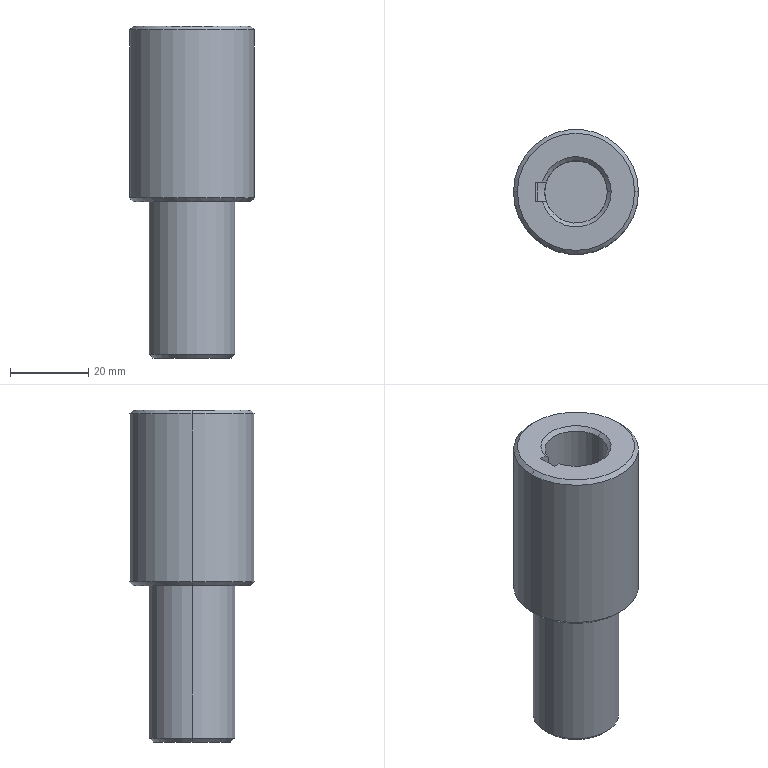Part | STEP file | HXGR200008-05-12-03 | 1 solid | 23 faces | box 32 x 32 x 85 mm | volume 43804 mm3 | cone 9 | plane 8 | cylinder 6 | commonest cylinder face diameters 16 x2 22 x2 32 x2
STEP:
#1=CARTESIAN_POINT('',(-10.,0.,0.));
#2=VERTEX_POINT('',#1);
#3=CARTESIAN_POINT('',(10.,0.,0.));
#4=VERTEX_POINT('',#3);
#5=CARTESIAN_POINT('',(0.,0.,0.));
#6=DIRECTION('',(0.,0.,-1.));
#7=DIRECTION('',(1.,0.,0.));
#8=AXIS2_PLACEMENT_3D('',#5,#6,#7);
#9=CIRCLE('',#8,10.);
#10=EDGE_CURVE('',#2,#4,#9,.T.);
#11=ORIENTED_EDGE('',*,*,#10,.F.);
#12=CARTESIAN_POINT('',(-11.,0.,1.));
#13=VERTEX_POINT('',#12);
#14=CARTESIAN_POINT('',(-11.,0.,1.));
#15=DIRECTION('',(-0.7071,0.,0.7071));
#16=VECTOR('',#15,1000.);
#17=LINE('',#14,#16);
#18=EDGE_CURVE('',#2,#13,#17,.T.);
#19=ORIENTED_EDGE('',*,*,#18,.T.);
#20=CARTESIAN_POINT('',(11.,0.,1.));
#21=VERTEX_POINT('',#20);
#22=CARTESIAN_POINT('',(0.,0.,1.));
#23=DIRECTION('',(0.,0.,1.));
#24=DIRECTION('',(1.,0.,0.));
#25=AXIS2_PLACEMENT_3D('',#22,#23,#24);
#26=CIRCLE('',#25,11.);
#27=EDGE_CURVE('',#21,#13,#26,.T.);
#28=ORIENTED_EDGE('',*,*,#27,.F.);
#29=CARTESIAN_POINT('',(11.,0.,1.));
#30=DIRECTION('',(0.7071,0.,0.7071));
#31=VECTOR('',#30,1000.);
#32=LINE('',#29,#31);
#33=EDGE_CURVE('',#4,#21,#32,.T.);
#34=ORIENTED_EDGE('',*,*,#33,.F.);
#35=EDGE_LOOP('',(#11,#19,#28,#34));
#36=FACE_OUTER_BOUND('',#35,.T.);
#37=CARTESIAN_POINT('',(0.,0.,1.));
#38=DIRECTION('',(0.,0.,1.));
#39=DIRECTION('',(1.,0.,0.));
#40=AXIS2_PLACEMENT_3D('',#37,#38,#39);
#41=CONICAL_SURFACE('',#40,11.,0.7854);
#42=ADVANCED_FACE('',(#36),#41,.T.);
#43=CARTESIAN_POINT('',(-15.,0.,40.));
#44=VERTEX_POINT('',#43);
#45=CARTESIAN_POINT('',(15.,0.,40.));
#46=VERTEX_POINT('',#45);
#47=CARTESIAN_POINT('',(0.,0.,40.));
#48=DIRECTION('',(0.,0.,-1.));
#49=DIRECTION('',(1.,0.,0.));
#50=AXIS2_PLACEMENT_3D('',#47,#48,#49);
#51=CIRCLE('',#50,15.);
#52=EDGE_CURVE('',#44,#46,#51,.T.);
#53=ORIENTED_EDGE('',*,*,#52,.F.);
#54=CARTESIAN_POINT('',(-16.,0.,41.));
#55=VERTEX_POINT('',#54);
#56=CARTESIAN_POINT('',(-16.,0.,41.));
#57=DIRECTION('',(-0.7071,0.,0.7071));
#58=VECTOR('',#57,1000.);
#59=LINE('',#56,#58);
#60=EDGE_CURVE('',#44,#55,#59,.T.);
#61=ORIENTED_EDGE('',*,*,#60,.T.);
#62=CARTESIAN_POINT('',(16.,0.,41.));
#63=VERTEX_POINT('',#62);
#64=CARTESIAN_POINT('',(0.,0.,41.));
#65=DIRECTION('',(0.,0.,1.));
#66=DIRECTION('',(1.,0.,0.));
#67=AXIS2_PLACEMENT_3D('',#64,#65,#66);
#68=CIRCLE('',#67,16.);
#69=EDGE_CURVE('',#63,#55,#68,.T.);
#70=ORIENTED_EDGE('',*,*,#69,.F.);
#71=CARTESIAN_POINT('',(16.,0.,41.));
#72=DIRECTION('',(0.7071,0.,0.7071));
#73=VECTOR('',#72,1000.);
#74=LINE('',#71,#73);
#75=EDGE_CURVE('',#46,#63,#74,.T.);
#76=ORIENTED_EDGE('',*,*,#75,.F.);
#77=EDGE_LOOP('',(#53,#61,#70,#76));
#78=FACE_OUTER_BOUND('',#77,.T.);
#79=CARTESIAN_POINT('',(0.,0.,41.));
#80=DIRECTION('',(0.,0.,1.));
#81=DIRECTION('',(1.,0.,0.));
#82=AXIS2_PLACEMENT_3D('',#79,#80,#81);
#83=CONICAL_SURFACE('',#82,16.,0.7854);
#84=ADVANCED_FACE('',(#78),#83,.T.);
#85=CARTESIAN_POINT('',(15.,0.,85.));
#86=VERTEX_POINT('',#85);
#87=CARTESIAN_POINT('',(-15.,0.,85.));
#88=VERTEX_POINT('',#87);
#89=CARTESIAN_POINT('',(0.,0.,85.));
#90=DIRECTION('',(0.,0.,1.));
#91=DIRECTION('',(1.,0.,0.));
#92=AXIS2_PLACEMENT_3D('',#89,#90,#91);
#93=CIRCLE('',#92,15.);
#94=EDGE_CURVE('',#86,#88,#93,.T.);
#95=ORIENTED_EDGE('',*,*,#94,.F.);
#96=CARTESIAN_POINT('',(16.,0.,84.));
#97=VERTEX_POINT('',#96);
#98=CARTESIAN_POINT('',(15.,0.,85.));
#99=DIRECTION('',(0.7071,0.,-0.7071));
#100=VECTOR('',#99,1000.);
#101=LINE('',#98,#100);
#102=EDGE_CURVE('',#86,#97,#101,.T.);
#103=ORIENTED_EDGE('',*,*,#102,.T.);
#104=CARTESIAN_POINT('',(-16.,0.,84.));
#105=VERTEX_POINT('',#104);
#106=CARTESIAN_POINT('',(0.,0.,84.));
#107=DIRECTION('',(0.,0.,-1.));
#108=DIRECTION('',(1.,0.,0.));
#109=AXIS2_PLACEMENT_3D('',#106,#107,#108);
#110=CIRCLE('',#109,16.);
#111=EDGE_CURVE('',#105,#97,#110,.T.);
#112=ORIENTED_EDGE('',*,*,#111,.F.);
#113=CARTESIAN_POINT('',(-15.,0.,85.));
#114=DIRECTION('',(-0.7071,0.,-0.7071));
#115=VECTOR('',#114,1000.);
#116=LINE('',#113,#115);
#117=EDGE_CURVE('',#88,#105,#116,.T.);
#118=ORIENTED_EDGE('',*,*,#117,.F.);
#119=EDGE_LOOP('',(#95,#103,#112,#118));
#120=FACE_OUTER_BOUND('',#119,.T.);
#121=CARTESIAN_POINT('',(0.,0.,85.));
#122=DIRECTION('',(0.,0.,-1.));
#123=DIRECTION('',(-1.,0.,0.));
#124=AXIS2_PLACEMENT_3D('',#121,#122,#123);
#125=CONICAL_SURFACE('',#124,15.,0.7854);
#126=ADVANCED_FACE('',(#120),#125,.T.);
#127=CARTESIAN_POINT('',(8.,0.,84.));
#128=VERTEX_POINT('',#127);
#129=CARTESIAN_POINT('',(-7.599,2.5,84.));
#130=VERTEX_POINT('',#129);
#131=CARTESIAN_POINT('',(0.,0.,84.));
#132=DIRECTION('',(0.,0.,1.));
#133=DIRECTION('',(1.,0.,0.));
#134=AXIS2_PLACEMENT_3D('',#131,#132,#133);
#135=CIRCLE('',#134,8.);
#136=EDGE_CURVE('',#128,#130,#135,.T.);
#137=ORIENTED_EDGE('',*,*,#136,.F.);
#138=CARTESIAN_POINT('',(9.,0.,85.));
#139=VERTEX_POINT('',#138);
#140=CARTESIAN_POINT('',(8.,0.,84.));
#141=DIRECTION('',(0.7071,0.,0.7071));
#142=VECTOR('',#141,1000.);
#143=LINE('',#140,#142);
#144=EDGE_CURVE('',#128,#139,#143,.T.);
#145=ORIENTED_EDGE('',*,*,#144,.T.);
#146=CARTESIAN_POINT('',(-8.646,2.5,85.));
#147=VERTEX_POINT('',#146);
#148=CARTESIAN_POINT('',(0.,0.,85.));
#149=DIRECTION('',(0.,0.,-1.));
#150=DIRECTION('',(1.,0.,0.));
#151=AXIS2_PLACEMENT_3D('',#148,#149,#150);
#152=CIRCLE('',#151,9.);
#153=EDGE_CURVE('',#147,#139,#152,.T.);
#154=ORIENTED_EDGE('',*,*,#153,.F.);
#155=CARTESIAN_POINT('',(-7.599,2.5,84.));
#156=CARTESIAN_POINT('',(-7.949,2.5,84.332));
#157=CARTESIAN_POINT('',(-8.298,2.5,84.666));
#158=CARTESIAN_POINT('',(-8.646,2.5,85.));
#159=B_SPLINE_CURVE_WITH_KNOTS('',3,(#155,#156,#157,#158),.UNSPECIFIED.,.F.,.F.,(4,4),(0.008066,0.009509),.UNSPECIFIED.);
#160=EDGE_CURVE('',#130,#147,#159,.T.);
#161=ORIENTED_EDGE('',*,*,#160,.F.);
#162=EDGE_LOOP('',(#137,#145,#154,#161));
#163=FACE_OUTER_BOUND('',#162,.T.);
#164=CARTESIAN_POINT('',(0.,0.,84.));
#165=DIRECTION('',(0.,0.,1.));
#166=DIRECTION('',(1.,0.,0.));
#167=AXIS2_PLACEMENT_3D('',#164,#165,#166);
#168=CONICAL_SURFACE('',#167,8.,0.7854);
#169=ADVANCED_FACE('',(#163),#168,.F.);
#170=CARTESIAN_POINT('',(-8.,0.,50.));
#171=VERTEX_POINT('',#170);
#172=CARTESIAN_POINT('',(8.,0.,50.));
#173=VERTEX_POINT('',#172);
#174=CARTESIAN_POINT('',(0.,0.,50.));
#175=DIRECTION('',(0.,0.,1.));
#176=DIRECTION('',(1.,0.,0.));
#177=AXIS2_PLACEMENT_3D('',#174,#175,#176);
#178=CIRCLE('',#177,8.);
#179=EDGE_CURVE('',#171,#173,#178,.T.);
#180=ORIENTED_EDGE('',*,*,#179,.F.);
#181=CARTESIAN_POINT('',(-8.,0.,51.));
#182=VERTEX_POINT('',#181);
#183=CARTESIAN_POINT('',(-8.,0.,50.));
#184=DIRECTION('',(0.,0.,1.));
#185=VECTOR('',#184,1000.);
#186=LINE('',#183,#185);
#187=EDGE_CURVE('',#171,#182,#186,.T.);
#188=ORIENTED_EDGE('',*,*,#187,.T.);
#189=CARTESIAN_POINT('',(-7.599,-2.5,51.));
#190=VERTEX_POINT('',#189);
#191=CARTESIAN_POINT('',(0.,0.,51.));
#192=DIRECTION('',(0.,0.,1.));
#193=DIRECTION('',(-1.,0.,0.));
#194=AXIS2_PLACEMENT_3D('',#191,#192,#193);
#195=CIRCLE('',#194,8.);
#196=EDGE_CURVE('',#182,#190,#195,.T.);
#197=ORIENTED_EDGE('',*,*,#196,.T.);
#198=CARTESIAN_POINT('',(-7.599,-2.5,84.));
#199=VERTEX_POINT('',#198);
#200=CARTESIAN_POINT('',(-7.599,-2.5,50.));
#201=DIRECTION('',(0.,0.,1.));
#202=VECTOR('',#201,1000.);
#203=LINE('',#200,#202);
#204=EDGE_CURVE('',#190,#199,#203,.T.);
#205=ORIENTED_EDGE('',*,*,#204,.T.);
#206=CARTESIAN_POINT('',(0.,0.,84.));
#207=DIRECTION('',(0.,0.,1.));
#208=DIRECTION('',(1.,0.,0.));
#209=AXIS2_PLACEMENT_3D('',#206,#207,#208);
#210=CIRCLE('',#209,8.);
#211=EDGE_CURVE('',#199,#128,#210,.T.);
#212=ORIENTED_EDGE('',*,*,#211,.T.);
#213=CARTESIAN_POINT('',(8.,0.,50.));
#214=DIRECTION('',(0.,0.,1.));
#215=VECTOR('',#214,1000.);
#216=LINE('',#213,#215);
#217=EDGE_CURVE('',#173,#128,#216,.T.);
#218=ORIENTED_EDGE('',*,*,#217,.F.);
#219=EDGE_LOOP('',(#180,#188,#197,#205,#212,#218));
#220=FACE_OUTER_BOUND('',#219,.T.);
#221=CARTESIAN_POINT('',(0.,0.,50.));
#222=DIRECTION('',(0.,0.,1.));
#223=DIRECTION('',(1.,0.,0.));
#224=AXIS2_PLACEMENT_3D('',#221,#222,#223);
#225=CYLINDRICAL_SURFACE('',#224,8.);
#226=ADVANCED_FACE('',(#220),#225,.F.);
#227=ORIENTED_EDGE('',*,*,#111,.T.);
#228=CARTESIAN_POINT('',(16.,0.,85.));
#229=DIRECTION('',(0.,0.,-1.));
#230=VECTOR('',#229,1000.);
#231=LINE('',#228,#230);
#232=EDGE_CURVE('',#97,#63,#231,.T.);
#233=ORIENTED_EDGE('',*,*,#232,.T.);
#234=ORIENTED_EDGE('',*,*,#69,.T.);
#235=CARTESIAN_POINT('',(-16.,0.,85.));
#236=DIRECTION('',(0.,0.,-1.));
#237=VECTOR('',#236,1000.);
#238=LINE('',#235,#237);
#239=EDGE_CURVE('',#105,#55,#238,.T.);
#240=ORIENTED_EDGE('',*,*,#239,.F.);
#241=EDGE_LOOP('',(#227,#233,#234,#240));
#242=FACE_OUTER_BOUND('',#241,.T.);
#243=CARTESIAN_POINT('',(0.,0.,85.));
#244=DIRECTION('',(0.,0.,-1.));
#245=DIRECTION('',(-1.,0.,0.));
#246=AXIS2_PLACEMENT_3D('',#243,#244,#245);
#247=CYLINDRICAL_SURFACE('',#246,16.);
#248=ADVANCED_FACE('',(#242),#247,.T.);
#249=CARTESIAN_POINT('',(11.,0.,40.));
#250=VERTEX_POINT('',#249);
#251=CARTESIAN_POINT('',(-11.,0.,40.));
#252=VERTEX_POINT('',#251);
#253=CARTESIAN_POINT('',(0.,0.,40.));
#254=DIRECTION('',(0.,0.,1.));
#255=DIRECTION('',(1.,0.,0.));
#256=AXIS2_PLACEMENT_3D('',#253,#254,#255);
#257=CIRCLE('',#256,11.);
#258=EDGE_CURVE('',#250,#252,#257,.T.);
#259=ORIENTED_EDGE('',*,*,#258,.F.);
#260=CARTESIAN_POINT('',(11.,0.,40.));
#261=DIRECTION('',(0.,0.,-1.));
#262=VECTOR('',#261,1000.);
#263=LINE('',#260,#262);
#264=EDGE_CURVE('',#250,#21,#263,.T.);
#265=ORIENTED_EDGE('',*,*,#264,.T.);
#266=ORIENTED_EDGE('',*,*,#27,.T.);
#267=CARTESIAN_POINT('',(-11.,0.,40.));
#268=DIRECTION('',(0.,0.,-1.));
#269=VECTOR('',#268,1000.);
#270=LINE('',#267,#269);
#271=EDGE_CURVE('',#252,#13,#270,.T.);
#272=ORIENTED_EDGE('',*,*,#271,.F.);
#273=EDGE_LOOP('',(#259,#265,#266,#272));
#274=FACE_OUTER_BOUND('',#273,.T.);
#275=CARTESIAN_POINT('',(0.,0.,40.));
#276=DIRECTION('',(0.,0.,-1.));
#277=DIRECTION('',(-1.,0.,0.));
#278=AXIS2_PLACEMENT_3D('',#275,#276,#277);
#279=CYLINDRICAL_SURFACE('',#278,11.);
#280=ADVANCED_FACE('',(#274),#279,.T.);
#281=ORIENTED_EDGE('',*,*,#264,.F.);
#282=CARTESIAN_POINT('',(0.,0.,40.));
#283=DIRECTION('',(0.,0.,1.));
#284=DIRECTION('',(1.,0.,0.));
#285=AXIS2_PLACEMENT_3D('',#282,#283,#284);
#286=CIRCLE('',#285,11.);
#287=EDGE_CURVE('',#252,#250,#286,.T.);
#288=ORIENTED_EDGE('',*,*,#287,.F.);
#289=ORIENTED_EDGE('',*,*,#271,.T.);
#290=CARTESIAN_POINT('',(0.,0.,1.));
#291=DIRECTION('',(0.,0.,1.));
#292=DIRECTION('',(1.,0.,0.));
#293=AXIS2_PLACEMENT_3D('',#290,#291,#292);
#294=CIRCLE('',#293,11.);
#295=EDGE_CURVE('',#13,#21,#294,.T.);
#296=ORIENTED_EDGE('',*,*,#295,.T.);
#297=EDGE_LOOP('',(#281,#288,#289,#296));
#298=FACE_OUTER_BOUND('',#297,.T.);
#299=CARTESIAN_POINT('',(0.,0.,40.));
#300=DIRECTION('',(0.,0.,-1.));
#301=DIRECTION('',(-1.,0.,0.));
#302=AXIS2_PLACEMENT_3D('',#299,#300,#301);
#303=CYLINDRICAL_SURFACE('',#302,11.);
#304=ADVANCED_FACE('',(#298),#303,.T.);
#305=CARTESIAN_POINT('',(0.,0.,0.));
#306=DIRECTION('',(0.,0.,-1.));
#307=DIRECTION('',(1.,0.,0.));
#308=AXIS2_PLACEMENT_3D('',#305,#306,#307);
#309=CIRCLE('',#308,10.);
#310=EDGE_CURVE('',#4,#2,#309,.T.);
#311=ORIENTED_EDGE('',*,*,#310,.T.);
#312=ORIENTED_EDGE('',*,*,#10,.T.);
#313=EDGE_LOOP('',(#311,#312));
#314=FACE_OUTER_BOUND('',#313,.T.);
#315=CARTESIAN_POINT('',(0.,0.,0.));
#316=DIRECTION('',(0.,0.,1.));
#317=DIRECTION('',(1.,0.,0.));
#318=AXIS2_PLACEMENT_3D('',#315,#316,#317);
#319=PLANE('',#318);
#320=ADVANCED_FACE('',(#314),#319,.F.);
#321=ORIENTED_EDGE('',*,*,#232,.F.);
#322=CARTESIAN_POINT('',(0.,0.,84.));
#323=DIRECTION('',(0.,0.,-1.));
#324=DIRECTION('',(1.,0.,0.));
#325=AXIS2_PLACEMENT_3D('',#322,#323,#324);
#326=CIRCLE('',#325,16.);
#327=EDGE_CURVE('',#97,#105,#326,.T.);
#328=ORIENTED_EDGE('',*,*,#327,.T.);
#329=ORIENTED_EDGE('',*,*,#239,.T.);
#330=CARTESIAN_POINT('',(0.,0.,41.));
#331=DIRECTION('',(0.,0.,1.));
#332=DIRECTION('',(1.,0.,0.));
#333=AXIS2_PLACEMENT_3D('',#330,#331,#332);
#334=CIRCLE('',#333,16.);
#335=EDGE_CURVE('',#55,#63,#334,.T.);
#336=ORIENTED_EDGE('',*,*,#335,.T.);
#337=EDGE_LOOP('',(#321,#328,#329,#336));
#338=FACE_OUTER_BOUND('',#337,.T.);
#339=CARTESIAN_POINT('',(0.,0.,85.));
#340=DIRECTION('',(0.,0.,-1.));
#341=DIRECTION('',(-1.,0.,0.));
#342=AXIS2_PLACEMENT_3D('',#339,#340,#341);
#343=CYLINDRICAL_SURFACE('',#342,16.);
#344=ADVANCED_FACE('',(#338),#343,.T.);
#345=CARTESIAN_POINT('',(-10.3,2.5,85.));
#346=VERTEX_POINT('',#345);
#347=CARTESIAN_POINT('',(-10.3,2.5,85.));
#348=DIRECTION('',(-1.,0.,0.));
#349=VECTOR('',#348,1000.);
#350=LINE('',#347,#349);
#351=EDGE_CURVE('',#147,#346,#350,.T.);
#352=ORIENTED_EDGE('',*,*,#351,.F.);
#353=ORIENTED_EDGE('',*,*,#153,.T.);
#354=CARTESIAN_POINT('',(-8.646,-2.5,85.));
#355=VERTEX_POINT('',#354);
#356=CARTESIAN_POINT('',(0.,0.,85.));
#357=DIRECTION('',(0.,0.,-1.));
#358=DIRECTION('',(1.,0.,0.));
#359=AXIS2_PLACEMENT_3D('',#356,#357,#358);
#360=CIRCLE('',#359,9.);
#361=EDGE_CURVE('',#139,#355,#360,.T.);
#362=ORIENTED_EDGE('',*,*,#361,.T.);
#363=CARTESIAN_POINT('',(-10.3,-2.5,85.));
#364=VERTEX_POINT('',#363);
#365=CARTESIAN_POINT('',(-10.3,-2.5,85.));
#366=DIRECTION('',(1.,0.,0.));
#367=VECTOR('',#366,1000.);
#368=LINE('',#365,#367);
#369=EDGE_CURVE('',#364,#355,#368,.T.);
#370=ORIENTED_EDGE('',*,*,#369,.F.);
#371=CARTESIAN_POINT('',(-10.3,-2.5,85.));
#372=DIRECTION('',(0.,-1.,0.));
#373=VECTOR('',#372,1000.);
#374=LINE('',#371,#373);
#375=EDGE_CURVE('',#346,#364,#374,.T.);
#376=ORIENTED_EDGE('',*,*,#375,.F.);
#377=EDGE_LOOP('',(#352,#353,#362,#370,#376));
#378=FACE_BOUND('',#377,.T.);
#379=CARTESIAN_POINT('',(0.,0.,85.));
#380=DIRECTION('',(0.,0.,1.));
#381=DIRECTION('',(1.,0.,0.));
#382=AXIS2_PLACEMENT_3D('',#379,#380,#381);
#383=CIRCLE('',#382,15.);
#384=EDGE_CURVE('',#88,#86,#383,.T.);
#385=ORIENTED_EDGE('',*,*,#384,.T.);
#386=ORIENTED_EDGE('',*,*,#94,.T.);
#387=EDGE_LOOP('',(#385,#386));
#388=FACE_OUTER_BOUND('',#387,.T.);
#389=CARTESIAN_POINT('',(0.,0.,85.));
#390=DIRECTION('',(0.,0.,1.));
#391=DIRECTION('',(1.,0.,0.));
#392=AXIS2_PLACEMENT_3D('',#389,#390,#391);
#393=PLANE('',#392);
#394=ADVANCED_FACE('',(#378,#388),#393,.T.);
#395=CARTESIAN_POINT('',(0.,0.,40.));
#396=DIRECTION('',(0.,0.,-1.));
#397=DIRECTION('',(1.,0.,0.));
#398=AXIS2_PLACEMENT_3D('',#395,#396,#397);
#399=CIRCLE('',#398,15.);
#400=EDGE_CURVE('',#46,#44,#399,.T.);
#401=ORIENTED_EDGE('',*,*,#400,.T.);
#402=ORIENTED_EDGE('',*,*,#52,.T.);
#403=EDGE_LOOP('',(#401,#402));
#404=FACE_OUTER_BOUND('',#403,.T.);
#405=ORIENTED_EDGE('',*,*,#287,.T.);
#406=ORIENTED_EDGE('',*,*,#258,.T.);
#407=EDGE_LOOP('',(#405,#406));
#408=FACE_BOUND('',#407,.T.);
#409=CARTESIAN_POINT('',(0.,0.,40.));
#410=DIRECTION('',(0.,0.,1.));
#411=DIRECTION('',(1.,0.,0.));
#412=AXIS2_PLACEMENT_3D('',#409,#410,#411);
#413=PLANE('',#412);
#414=ADVANCED_FACE('',(#404,#408),#413,.F.);
#415=ORIENTED_EDGE('',*,*,#187,.F.);
#416=CARTESIAN_POINT('',(0.,0.,50.));
#417=DIRECTION('',(0.,0.,1.));
#418=DIRECTION('',(1.,0.,0.));
#419=AXIS2_PLACEMENT_3D('',#416,#417,#418);
#420=CIRCLE('',#419,8.);
#421=EDGE_CURVE('',#173,#171,#420,.T.);
#422=ORIENTED_EDGE('',*,*,#421,.F.);
#423=ORIENTED_EDGE('',*,*,#217,.T.);
#424=ORIENTED_EDGE('',*,*,#136,.T.);
#425=CARTESIAN_POINT('',(-7.599,2.5,51.));
#426=VERTEX_POINT('',#425);
#427=CARTESIAN_POINT('',(-7.599,2.5,50.));
#428=DIRECTION('',(0.,0.,-1.));
#429=VECTOR('',#428,1000.);
#430=LINE('',#427,#429);
#431=EDGE_CURVE('',#130,#426,#430,.T.);
#432=ORIENTED_EDGE('',*,*,#431,.T.);
#433=CARTESIAN_POINT('',(0.,0.,51.));
#434=DIRECTION('',(0.,0.,1.));
#435=DIRECTION('',(-1.,0.,0.));
#436=AXIS2_PLACEMENT_3D('',#433,#434,#435);
#437=CIRCLE('',#436,8.);
#438=EDGE_CURVE('',#426,#182,#437,.T.);
#439=ORIENTED_EDGE('',*,*,#438,.T.);
#440=EDGE_LOOP('',(#415,#422,#423,#424,#432,#439));
#441=FACE_OUTER_BOUND('',#440,.T.);
#442=CARTESIAN_POINT('',(0.,0.,50.));
#443=DIRECTION('',(0.,0.,1.));
#444=DIRECTION('',(1.,0.,0.));
#445=AXIS2_PLACEMENT_3D('',#442,#443,#444);
#446=CYLINDRICAL_SURFACE('',#445,8.);
#447=ADVANCED_FACE('',(#441),#446,.F.);
#448=ORIENTED_EDGE('',*,*,#421,.T.);
#449=ORIENTED_EDGE('',*,*,#179,.T.);
#450=EDGE_LOOP('',(#448,#449));
#451=FACE_OUTER_BOUND('',#450,.T.);
#452=CARTESIAN_POINT('',(0.,0.,50.));
#453=DIRECTION('',(0.,0.,1.));
#454=DIRECTION('',(1.,0.,0.));
#455=AXIS2_PLACEMENT_3D('',#452,#453,#454);
#456=PLANE('',#455);
#457=ADVANCED_FACE('',(#451),#456,.T.);
#458=ORIENTED_EDGE('',*,*,#144,.F.);
#459=ORIENTED_EDGE('',*,*,#211,.F.);
#460=CARTESIAN_POINT('',(-8.646,-2.5,85.));
#461=CARTESIAN_POINT('',(-8.298,-2.5,84.666));
#462=CARTESIAN_POINT('',(-7.949,-2.5,84.332));
#463=CARTESIAN_POINT('',(-7.599,-2.5,84.));
#464=B_SPLINE_CURVE_WITH_KNOTS('',3,(#460,#461,#462,#463),.UNSPECIFIED.,.F.,.F.,(4,4),(0.008462,0.00991),.UNSPECIFIED.);
#465=EDGE_CURVE('',#355,#199,#464,.T.);
#466=ORIENTED_EDGE('',*,*,#465,.F.);
#467=ORIENTED_EDGE('',*,*,#361,.F.);
#468=EDGE_LOOP('',(#458,#459,#466,#467));
#469=FACE_OUTER_BOUND('',#468,.T.);
#470=CARTESIAN_POINT('',(0.,0.,84.));
#471=DIRECTION('',(0.,0.,1.));
#472=DIRECTION('',(1.,0.,0.));
#473=AXIS2_PLACEMENT_3D('',#470,#471,#472);
#474=CONICAL_SURFACE('',#473,8.,0.7854);
#475=ADVANCED_FACE('',(#469),#474,.F.);
#476=ORIENTED_EDGE('',*,*,#102,.F.);
#477=ORIENTED_EDGE('',*,*,#384,.F.);
#478=ORIENTED_EDGE('',*,*,#117,.T.);
#479=ORIENTED_EDGE('',*,*,#327,.F.);
#480=EDGE_LOOP('',(#476,#477,#478,#479));
#481=FACE_OUTER_BOUND('',#480,.T.);
#482=CARTESIAN_POINT('',(0.,0.,85.));
#483=DIRECTION('',(0.,0.,-1.));
#484=DIRECTION('',(-1.,0.,0.));
#485=AXIS2_PLACEMENT_3D('',#482,#483,#484);
#486=CONICAL_SURFACE('',#485,15.,0.7854);
#487=ADVANCED_FACE('',(#481),#486,.T.);
#488=ORIENTED_EDGE('',*,*,#60,.F.);
#489=ORIENTED_EDGE('',*,*,#400,.F.);
#490=ORIENTED_EDGE('',*,*,#75,.T.);
#491=ORIENTED_EDGE('',*,*,#335,.F.);
#492=EDGE_LOOP('',(#488,#489,#490,#491));
#493=FACE_OUTER_BOUND('',#492,.T.);
#494=CARTESIAN_POINT('',(0.,0.,41.));
#495=DIRECTION('',(0.,0.,1.));
#496=DIRECTION('',(1.,0.,0.));
#497=AXIS2_PLACEMENT_3D('',#494,#495,#496);
#498=CONICAL_SURFACE('',#497,16.,0.7854);
#499=ADVANCED_FACE('',(#493),#498,.T.);
#500=ORIENTED_EDGE('',*,*,#18,.F.);
#501=ORIENTED_EDGE('',*,*,#310,.F.);
#502=ORIENTED_EDGE('',*,*,#33,.T.);
#503=ORIENTED_EDGE('',*,*,#295,.F.);
#504=EDGE_LOOP('',(#500,#501,#502,#503));
#505=FACE_OUTER_BOUND('',#504,.T.);
#506=CARTESIAN_POINT('',(0.,0.,1.));
#507=DIRECTION('',(0.,0.,1.));
#508=DIRECTION('',(1.,0.,0.));
#509=AXIS2_PLACEMENT_3D('',#506,#507,#508);
#510=CONICAL_SURFACE('',#509,11.,0.7854);
#511=ADVANCED_FACE('',(#505),#510,.T.);
#512=CARTESIAN_POINT('',(-10.3,-2.5,53.));
#513=VERTEX_POINT('',#512);
#514=CARTESIAN_POINT('',(-9.682,-2.5,53.));
#515=VERTEX_POINT('',#514);
#516=CARTESIAN_POINT('',(-10.3,-2.5,53.));
#517=DIRECTION('',(1.,0.,0.));
#518=VECTOR('',#517,1000.);
#519=LINE('',#516,#518);
#520=EDGE_CURVE('',#513,#515,#519,.T.);
#521=ORIENTED_EDGE('',*,*,#520,.T.);
#522=CARTESIAN_POINT('',(-9.682,2.5,53.));
#523=VERTEX_POINT('',#522);
#524=CARTESIAN_POINT('',(0.,0.,53.));
#525=DIRECTION('',(0.,0.,-1.));
#526=DIRECTION('',(-1.,0.,0.));
#527=AXIS2_PLACEMENT_3D('',#524,#525,#526);
#528=CIRCLE('',#527,10.);
#529=EDGE_CURVE('',#515,#523,#528,.T.);
#530=ORIENTED_EDGE('',*,*,#529,.T.);
#531=CARTESIAN_POINT('',(-10.3,2.5,53.));
#532=VERTEX_POINT('',#531);
#533=CARTESIAN_POINT('',(-10.3,2.5,53.));
#534=DIRECTION('',(-1.,0.,0.));
#535=VECTOR('',#534,1000.);
#536=LINE('',#533,#535);
#537=EDGE_CURVE('',#523,#532,#536,.T.);
#538=ORIENTED_EDGE('',*,*,#537,.T.);
#539=CARTESIAN_POINT('',(-10.3,-2.5,53.));
#540=DIRECTION('',(0.,-1.,0.));
#541=VECTOR('',#540,1000.);
#542=LINE('',#539,#541);
#543=EDGE_CURVE('',#532,#513,#542,.T.);
#544=ORIENTED_EDGE('',*,*,#543,.T.);
#545=EDGE_LOOP('',(#521,#530,#538,#544));
#546=FACE_OUTER_BOUND('',#545,.T.);
#547=CARTESIAN_POINT('',(0.,0.,53.));
#548=DIRECTION('',(0.,0.,-1.));
#549=DIRECTION('',(-1.,0.,0.));
#550=AXIS2_PLACEMENT_3D('',#547,#548,#549);
#551=PLANE('',#550);
#552=ADVANCED_FACE('',(#546),#551,.F.);
#553=ORIENTED_EDGE('',*,*,#160,.T.);
#554=ORIENTED_EDGE('',*,*,#351,.T.);
#555=CARTESIAN_POINT('',(-10.3,2.5,53.));
#556=DIRECTION('',(0.,0.,1.));
#557=VECTOR('',#556,1000.);
#558=LINE('',#555,#557);
#559=EDGE_CURVE('',#532,#346,#558,.T.);
#560=ORIENTED_EDGE('',*,*,#559,.F.);
#561=ORIENTED_EDGE('',*,*,#537,.F.);
#562=CARTESIAN_POINT('',(-9.682,2.5,53.));
#563=CARTESIAN_POINT('',(-8.991,2.5,52.33));
#564=CARTESIAN_POINT('',(-8.297,2.5,51.663));
#565=CARTESIAN_POINT('',(-7.599,2.5,51.));
#566=B_SPLINE_CURVE_WITH_KNOTS('',3,(#562,#563,#564,#565),.UNSPECIFIED.,.F.,.F.,(4,4),(0.,0.002888),.UNSPECIFIED.);
#567=EDGE_CURVE('',#523,#426,#566,.T.);
#568=ORIENTED_EDGE('',*,*,#567,.T.);
#569=ORIENTED_EDGE('',*,*,#431,.F.);
#570=EDGE_LOOP('',(#553,#554,#560,#561,#568,#569));
#571=FACE_OUTER_BOUND('',#570,.T.);
#572=CARTESIAN_POINT('',(-10.3,2.5,53.));
#573=DIRECTION('',(0.,1.,0.));
#574=DIRECTION('',(0.,0.,1.));
#575=AXIS2_PLACEMENT_3D('',#572,#573,#574);
#576=PLANE('',#575);
#577=ADVANCED_FACE('',(#571),#576,.F.);
#578=ORIENTED_EDGE('',*,*,#520,.F.);
#579=CARTESIAN_POINT('',(-10.3,-2.5,53.));
#580=DIRECTION('',(0.,0.,1.));
#581=VECTOR('',#580,1000.);
#582=LINE('',#579,#581);
#583=EDGE_CURVE('',#513,#364,#582,.T.);
#584=ORIENTED_EDGE('',*,*,#583,.T.);
#585=ORIENTED_EDGE('',*,*,#369,.T.);
#586=ORIENTED_EDGE('',*,*,#465,.T.);
#587=ORIENTED_EDGE('',*,*,#204,.F.);
#588=CARTESIAN_POINT('',(-7.599,-2.5,51.));
#589=CARTESIAN_POINT('',(-8.297,-2.5,51.663));
#590=CARTESIAN_POINT('',(-8.991,-2.5,52.33));
#591=CARTESIAN_POINT('',(-9.682,-2.5,53.));
#592=B_SPLINE_CURVE_WITH_KNOTS('',3,(#588,#589,#590,#591),.UNSPECIFIED.,.F.,.F.,(4,4),(0.,0.002888),.UNSPECIFIED.);
#593=EDGE_CURVE('',#190,#515,#592,.T.);
#594=ORIENTED_EDGE('',*,*,#593,.T.);
#595=EDGE_LOOP('',(#578,#584,#585,#586,#587,#594));
#596=FACE_OUTER_BOUND('',#595,.T.);
#597=CARTESIAN_POINT('',(-10.3,-2.5,53.));
#598=DIRECTION('',(0.,-1.,0.));
#599=DIRECTION('',(0.,0.,-1.));
#600=AXIS2_PLACEMENT_3D('',#597,#598,#599);
#601=PLANE('',#600);
#602=ADVANCED_FACE('',(#596),#601,.F.);
#603=ORIENTED_EDGE('',*,*,#375,.T.);
#604=ORIENTED_EDGE('',*,*,#583,.F.);
#605=ORIENTED_EDGE('',*,*,#543,.F.);
#606=ORIENTED_EDGE('',*,*,#559,.T.);
#607=EDGE_LOOP('',(#603,#604,#605,#606));
#608=FACE_OUTER_BOUND('',#607,.T.);
#609=CARTESIAN_POINT('',(-10.3,-2.5,53.));
#610=DIRECTION('',(-1.,0.,0.));
#611=DIRECTION('',(0.,0.,1.));
#612=AXIS2_PLACEMENT_3D('',#609,#610,#611);
#613=PLANE('',#612);
#614=ADVANCED_FACE('',(#608),#613,.F.);
#615=ORIENTED_EDGE('',*,*,#567,.F.);
#616=ORIENTED_EDGE('',*,*,#529,.F.);
#617=ORIENTED_EDGE('',*,*,#593,.F.);
#618=ORIENTED_EDGE('',*,*,#196,.F.);
#619=ORIENTED_EDGE('',*,*,#438,.F.);
#620=EDGE_LOOP('',(#615,#616,#617,#618,#619));
#621=FACE_OUTER_BOUND('',#620,.T.);
#622=CARTESIAN_POINT('',(0.,0.,51.));
#623=DIRECTION('',(0.,0.,1.));
#624=DIRECTION('',(1.,0.,0.));
#625=AXIS2_PLACEMENT_3D('',#622,#623,#624);
#626=CONICAL_SURFACE('',#625,8.,0.7854);
#627=ADVANCED_FACE('',(#621),#626,.F.);
#628=CLOSED_SHELL('',(#42,#84,#126,#169,#226,#248,#280,#304,#320,#344,#394,#414,#447,#457,#475,#487,#499,#511,#552,#577,#602,#614,#627));
#629=MANIFOLD_SOLID_BREP('',#628);
#630=CARTESIAN_POINT('',(0.,0.,0.));
#631=DIRECTION('',(0.,0.,1.));
#632=DIRECTION('',(1.,0.,0.));
#633=AXIS2_PLACEMENT_3D('',#630,#631,#632);
#634=(LENGTH_UNIT()NAMED_UNIT(*)SI_UNIT(.MILLI.,.METRE.));
#635=UNCERTAINTY_MEASURE_WITH_UNIT(LENGTH_MEASURE(0.00001),#634,'','');
#636=(NAMED_UNIT(*)PLANE_ANGLE_UNIT()SI_UNIT($,.RADIAN.));
#637=(NAMED_UNIT(*)SI_UNIT($,.STERADIAN.)SOLID_ANGLE_UNIT());
#638=(GEOMETRIC_REPRESENTATION_CONTEXT(3)GLOBAL_UNCERTAINTY_ASSIGNED_CONTEXT((#635))GLOBAL_UNIT_ASSIGNED_CONTEXT((#634,#636,#637))REPRESENTATION_CONTEXT('',''));
#639=ADVANCED_BREP_SHAPE_REPRESENTATION('',(#629,#633),#638);